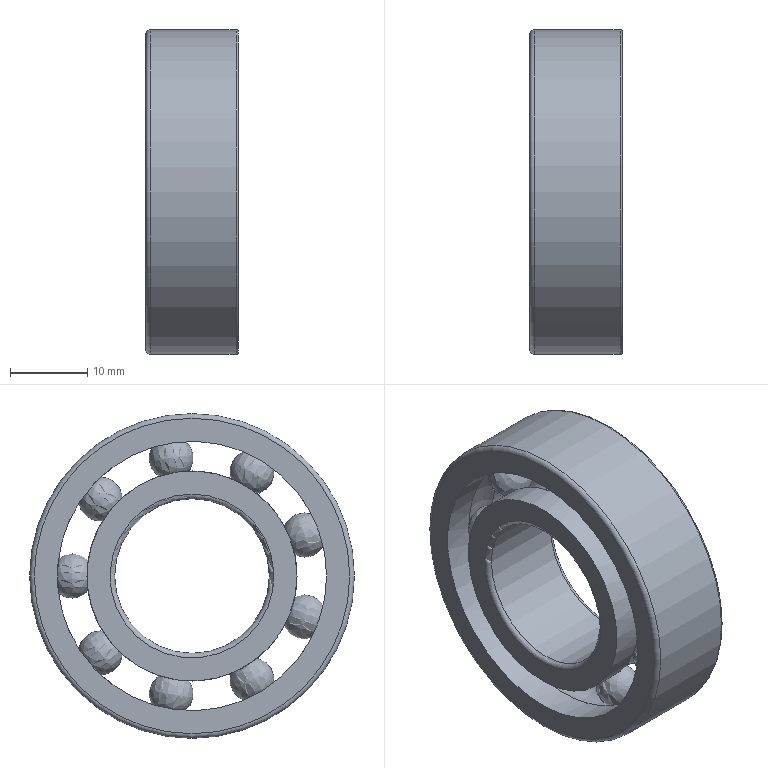Part | STEP file | Rolling bearing 70000C 7004 C GB_T 292 | 11 solids | 41 faces | box 12 x 42 x 42 mm | volume 8552 mm3 | torus 22 | sphere 9 | cylinder 5 | plane 4 | cone 1 | commonest cylinder face diameters 27.172 x2 20 x1 34.828 x1 42 x1
STEP:
#1=CARTESIAN_POINT('',(6.,13.712,-7.772));
#2=VERTEX_POINT('',#1);
#3=CARTESIAN_POINT('',(6.,10.035,-12.154));
#4=VERTEX_POINT('',#3);
#5=CARTESIAN_POINT('',(6.,11.874,-9.963));
#6=DIRECTION('',(0.,-0.766,0.6428));
#7=DIRECTION('',(-1.,0.,0.));
#8=AXIS2_PLACEMENT_3D('',#5,#6,#7);
#9=CIRCLE('',#8,2.86);
#10=EDGE_CURVE('',#2,#4,#9,.T.);
#11=ORIENTED_EDGE('',*,*,#10,.T.);
#12=ORIENTED_EDGE('',*,*,#10,.F.);
#13=EDGE_LOOP('',(#11,#12));
#14=FACE_OUTER_BOUND('',#13,.T.);
#15=CARTESIAN_POINT('',(3.875,10.407,-8.733));
#16=VERTEX_POINT('',#15);
#17=CARTESIAN_POINT('',(8.125,10.407,-8.733));
#18=VERTEX_POINT('',#17);
#19=CARTESIAN_POINT('',(6.,11.874,-9.963));
#20=DIRECTION('',(0.,0.6428,0.766));
#21=DIRECTION('',(0.,0.766,-0.6428));
#22=AXIS2_PLACEMENT_3D('',#19,#20,#21);
#23=CIRCLE('',#22,2.86);
#24=EDGE_CURVE('',#16,#18,#23,.T.);
#25=ORIENTED_EDGE('',*,*,#24,.T.);
#26=ORIENTED_EDGE('',*,*,#24,.F.);
#27=EDGE_LOOP('',(#25,#26));
#28=FACE_BOUND('',#27,.T.);
#29=CARTESIAN_POINT('',(8.125,13.34,-11.194));
#30=VERTEX_POINT('',#29);
#31=CARTESIAN_POINT('',(3.875,13.34,-11.194));
#32=VERTEX_POINT('',#31);
#33=CARTESIAN_POINT('',(6.,11.874,-9.963));
#34=DIRECTION('',(0.,0.6428,0.766));
#35=DIRECTION('',(0.,0.766,-0.6428));
#36=AXIS2_PLACEMENT_3D('',#33,#34,#35);
#37=CIRCLE('',#36,2.86);
#38=EDGE_CURVE('',#30,#32,#37,.T.);
#39=ORIENTED_EDGE('',*,*,#38,.T.);
#40=ORIENTED_EDGE('',*,*,#38,.F.);
#41=EDGE_LOOP('',(#39,#40));
#42=FACE_BOUND('',#41,.T.);
#43=CARTESIAN_POINT('',(6.,11.874,-9.963));
#44=DIRECTION('',(0.,0.6428,0.766));
#45=DIRECTION('',(1.,0.,0.));
#46=AXIS2_PLACEMENT_3D('',#43,#44,#45);
#47=SPHERICAL_SURFACE('',#46,2.86);
#48=ADVANCED_FACE('',(#14,#28,#42),#47,.T.);
#49=CLOSED_SHELL('',(#48));
#50=MANIFOLD_SOLID_BREP('',#49);
#51=CARTESIAN_POINT('',(6.,-10.227,11.993));
#52=VERTEX_POINT('',#51);
#53=CARTESIAN_POINT('',(6.,-5.273,14.853));
#54=VERTEX_POINT('',#53);
#55=CARTESIAN_POINT('',(6.,-7.75,13.423));
#56=DIRECTION('',(0.,0.5,-0.866));
#57=DIRECTION('',(-1.,0.,0.));
#58=AXIS2_PLACEMENT_3D('',#55,#56,#57);
#59=CIRCLE('',#58,2.86);
#60=EDGE_CURVE('',#52,#54,#59,.T.);
#61=ORIENTED_EDGE('',*,*,#60,.T.);
#62=ORIENTED_EDGE('',*,*,#60,.F.);
#63=EDGE_LOOP('',(#61,#62));
#64=FACE_OUTER_BOUND('',#63,.T.);
#65=CARTESIAN_POINT('',(3.875,-6.793,11.766));
#66=VERTEX_POINT('',#65);
#67=CARTESIAN_POINT('',(8.125,-6.793,11.766));
#68=VERTEX_POINT('',#67);
#69=CARTESIAN_POINT('',(6.,-7.75,13.423));
#70=DIRECTION('',(0.,-0.866,-0.5));
#71=DIRECTION('',(0.,-0.5,0.866));
#72=AXIS2_PLACEMENT_3D('',#69,#70,#71);
#73=CIRCLE('',#72,2.86);
#74=EDGE_CURVE('',#66,#68,#73,.T.);
#75=ORIENTED_EDGE('',*,*,#74,.T.);
#76=ORIENTED_EDGE('',*,*,#74,.F.);
#77=EDGE_LOOP('',(#75,#76));
#78=FACE_BOUND('',#77,.T.);
#79=CARTESIAN_POINT('',(8.125,-8.707,15.081));
#80=VERTEX_POINT('',#79);
#81=CARTESIAN_POINT('',(3.875,-8.707,15.081));
#82=VERTEX_POINT('',#81);
#83=CARTESIAN_POINT('',(6.,-7.75,13.423));
#84=DIRECTION('',(0.,-0.866,-0.5));
#85=DIRECTION('',(0.,-0.5,0.866));
#86=AXIS2_PLACEMENT_3D('',#83,#84,#85);
#87=CIRCLE('',#86,2.86);
#88=EDGE_CURVE('',#80,#82,#87,.T.);
#89=ORIENTED_EDGE('',*,*,#88,.T.);
#90=ORIENTED_EDGE('',*,*,#88,.F.);
#91=EDGE_LOOP('',(#89,#90));
#92=FACE_BOUND('',#91,.T.);
#93=CARTESIAN_POINT('',(6.,-7.75,13.423));
#94=DIRECTION('',(0.,-0.866,-0.5));
#95=DIRECTION('',(1.,0.,0.));
#96=AXIS2_PLACEMENT_3D('',#93,#94,#95);
#97=SPHERICAL_SURFACE('',#96,2.86);
#98=ADVANCED_FACE('',(#64,#78,#92),#97,.T.);
#99=CLOSED_SHELL('',(#98));
#100=MANIFOLD_SOLID_BREP('',#99);
#101=CARTESIAN_POINT('',(6.,-0.125,15.761));
#102=VERTEX_POINT('',#101);
#103=CARTESIAN_POINT('',(6.,5.508,14.768));
#104=VERTEX_POINT('',#103);
#105=CARTESIAN_POINT('',(6.,2.692,15.265));
#106=DIRECTION('',(0.,-0.1736,-0.9848));
#107=DIRECTION('',(-1.,0.,0.));
#108=AXIS2_PLACEMENT_3D('',#105,#106,#107);
#109=CIRCLE('',#108,2.86);
#110=EDGE_CURVE('',#102,#104,#109,.T.);
#111=ORIENTED_EDGE('',*,*,#110,.T.);
#112=ORIENTED_EDGE('',*,*,#110,.F.);
#113=EDGE_LOOP('',(#111,#112));
#114=FACE_OUTER_BOUND('',#113,.T.);
#115=CARTESIAN_POINT('',(3.875,2.359,13.38));
#116=VERTEX_POINT('',#115);
#117=CARTESIAN_POINT('',(8.125,2.359,13.38));
#118=VERTEX_POINT('',#117);
#119=CARTESIAN_POINT('',(6.,2.692,15.265));
#120=DIRECTION('',(0.,-0.9848,0.1736));
#121=DIRECTION('',(0.,0.1736,0.9848));
#122=AXIS2_PLACEMENT_3D('',#119,#120,#121);
#123=CIRCLE('',#122,2.86);
#124=EDGE_CURVE('',#116,#118,#123,.T.);
#125=ORIENTED_EDGE('',*,*,#124,.T.);
#126=ORIENTED_EDGE('',*,*,#124,.F.);
#127=EDGE_LOOP('',(#125,#126));
#128=FACE_BOUND('',#127,.T.);
#129=CARTESIAN_POINT('',(8.125,3.024,17.149));
#130=VERTEX_POINT('',#129);
#131=CARTESIAN_POINT('',(3.875,3.024,17.149));
#132=VERTEX_POINT('',#131);
#133=CARTESIAN_POINT('',(6.,2.692,15.265));
#134=DIRECTION('',(0.,-0.9848,0.1736));
#135=DIRECTION('',(0.,0.1736,0.9848));
#136=AXIS2_PLACEMENT_3D('',#133,#134,#135);
#137=CIRCLE('',#136,2.86);
#138=EDGE_CURVE('',#130,#132,#137,.T.);
#139=ORIENTED_EDGE('',*,*,#138,.T.);
#140=ORIENTED_EDGE('',*,*,#138,.F.);
#141=EDGE_LOOP('',(#139,#140));
#142=FACE_BOUND('',#141,.T.);
#143=CARTESIAN_POINT('',(6.,2.692,15.265));
#144=DIRECTION('',(0.,-0.9848,0.1736));
#145=DIRECTION('',(1.,0.,0.));
#146=AXIS2_PLACEMENT_3D('',#143,#144,#145);
#147=SPHERICAL_SURFACE('',#146,2.86);
#148=ADVANCED_FACE('',(#114,#128,#142),#147,.T.);
#149=CLOSED_SHELL('',(#148));
#150=MANIFOLD_SOLID_BREP('',#149);
#151=CARTESIAN_POINT('',(6.,-15.543,2.614));
#152=VERTEX_POINT('',#151);
#153=CARTESIAN_POINT('',(6.,-13.587,7.989));
#154=VERTEX_POINT('',#153);
#155=CARTESIAN_POINT('',(6.,-14.565,5.301));
#156=DIRECTION('',(0.,0.9397,-0.342));
#157=DIRECTION('',(-1.,0.,0.));
#158=AXIS2_PLACEMENT_3D('',#155,#156,#157);
#159=CIRCLE('',#158,2.86);
#160=EDGE_CURVE('',#152,#154,#159,.T.);
#161=ORIENTED_EDGE('',*,*,#160,.T.);
#162=ORIENTED_EDGE('',*,*,#160,.F.);
#163=EDGE_LOOP('',(#161,#162));
#164=FACE_OUTER_BOUND('',#163,.T.);
#165=CARTESIAN_POINT('',(3.875,-12.767,4.647));
#166=VERTEX_POINT('',#165);
#167=CARTESIAN_POINT('',(8.125,-12.767,4.647));
#168=VERTEX_POINT('',#167);
#169=CARTESIAN_POINT('',(6.,-14.565,5.301));
#170=DIRECTION('',(0.,-0.342,-0.9397));
#171=DIRECTION('',(0.,-0.9397,0.342));
#172=AXIS2_PLACEMENT_3D('',#169,#170,#171);
#173=CIRCLE('',#172,2.86);
#174=EDGE_CURVE('',#166,#168,#173,.T.);
#175=ORIENTED_EDGE('',*,*,#174,.T.);
#176=ORIENTED_EDGE('',*,*,#174,.F.);
#177=EDGE_LOOP('',(#175,#176));
#178=FACE_BOUND('',#177,.T.);
#179=CARTESIAN_POINT('',(8.125,-16.364,5.956));
#180=VERTEX_POINT('',#179);
#181=CARTESIAN_POINT('',(3.875,-16.364,5.956));
#182=VERTEX_POINT('',#181);
#183=CARTESIAN_POINT('',(6.,-14.565,5.301));
#184=DIRECTION('',(0.,-0.342,-0.9397));
#185=DIRECTION('',(0.,-0.9397,0.342));
#186=AXIS2_PLACEMENT_3D('',#183,#184,#185);
#187=CIRCLE('',#186,2.86);
#188=EDGE_CURVE('',#180,#182,#187,.T.);
#189=ORIENTED_EDGE('',*,*,#188,.T.);
#190=ORIENTED_EDGE('',*,*,#188,.F.);
#191=EDGE_LOOP('',(#189,#190));
#192=FACE_BOUND('',#191,.T.);
#193=CARTESIAN_POINT('',(6.,-14.565,5.301));
#194=DIRECTION('',(0.,-0.342,-0.9397));
#195=DIRECTION('',(1.,0.,0.));
#196=AXIS2_PLACEMENT_3D('',#193,#194,#195);
#197=SPHERICAL_SURFACE('',#196,2.86);
#198=ADVANCED_FACE('',(#164,#178,#192),#197,.T.);
#199=CLOSED_SHELL('',(#198));
#200=MANIFOLD_SOLID_BREP('',#199);
#201=CARTESIAN_POINT('',(6.,10.035,12.154));
#202=VERTEX_POINT('',#201);
#203=CARTESIAN_POINT('',(6.,13.712,7.772));
#204=VERTEX_POINT('',#203);
#205=CARTESIAN_POINT('',(6.,11.874,9.963));
#206=DIRECTION('',(0.,-0.766,-0.6428));
#207=DIRECTION('',(-1.,0.,0.));
#208=AXIS2_PLACEMENT_3D('',#205,#206,#207);
#209=CIRCLE('',#208,2.86);
#210=EDGE_CURVE('',#202,#204,#209,.T.);
#211=ORIENTED_EDGE('',*,*,#210,.T.);
#212=ORIENTED_EDGE('',*,*,#210,.F.);
#213=EDGE_LOOP('',(#211,#212));
#214=FACE_OUTER_BOUND('',#213,.T.);
#215=CARTESIAN_POINT('',(3.875,10.407,8.733));
#216=VERTEX_POINT('',#215);
#217=CARTESIAN_POINT('',(8.125,10.407,8.733));
#218=VERTEX_POINT('',#217);
#219=CARTESIAN_POINT('',(6.,11.874,9.963));
#220=DIRECTION('',(0.,-0.6428,0.766));
#221=DIRECTION('',(0.,0.766,0.6428));
#222=AXIS2_PLACEMENT_3D('',#219,#220,#221);
#223=CIRCLE('',#222,2.86);
#224=EDGE_CURVE('',#216,#218,#223,.T.);
#225=ORIENTED_EDGE('',*,*,#224,.T.);
#226=ORIENTED_EDGE('',*,*,#224,.F.);
#227=EDGE_LOOP('',(#225,#226));
#228=FACE_BOUND('',#227,.T.);
#229=CARTESIAN_POINT('',(8.125,13.34,11.194));
#230=VERTEX_POINT('',#229);
#231=CARTESIAN_POINT('',(3.875,13.34,11.194));
#232=VERTEX_POINT('',#231);
#233=CARTESIAN_POINT('',(6.,11.874,9.963));
#234=DIRECTION('',(0.,-0.6428,0.766));
#235=DIRECTION('',(0.,0.766,0.6428));
#236=AXIS2_PLACEMENT_3D('',#233,#234,#235);
#237=CIRCLE('',#236,2.86);
#238=EDGE_CURVE('',#230,#232,#237,.T.);
#239=ORIENTED_EDGE('',*,*,#238,.T.);
#240=ORIENTED_EDGE('',*,*,#238,.F.);
#241=EDGE_LOOP('',(#239,#240));
#242=FACE_BOUND('',#241,.T.);
#243=CARTESIAN_POINT('',(6.,11.874,9.963));
#244=DIRECTION('',(0.,-0.6428,0.766));
#245=DIRECTION('',(1.,0.,0.));
#246=AXIS2_PLACEMENT_3D('',#243,#244,#245);
#247=SPHERICAL_SURFACE('',#246,2.86);
#248=ADVANCED_FACE('',(#214,#228,#242),#247,.T.);
#249=CLOSED_SHELL('',(#248));
#250=MANIFOLD_SOLID_BREP('',#249);
#251=CARTESIAN_POINT('',(6.,-13.587,-7.989));
#252=VERTEX_POINT('',#251);
#253=CARTESIAN_POINT('',(6.,-15.543,-2.614));
#254=VERTEX_POINT('',#253);
#255=CARTESIAN_POINT('',(6.,-14.565,-5.301));
#256=DIRECTION('',(0.,0.9397,0.342));
#257=DIRECTION('',(-1.,0.,0.));
#258=AXIS2_PLACEMENT_3D('',#255,#256,#257);
#259=CIRCLE('',#258,2.86);
#260=EDGE_CURVE('',#252,#254,#259,.T.);
#261=ORIENTED_EDGE('',*,*,#260,.T.);
#262=ORIENTED_EDGE('',*,*,#260,.F.);
#263=EDGE_LOOP('',(#261,#262));
#264=FACE_OUTER_BOUND('',#263,.T.);
#265=CARTESIAN_POINT('',(3.875,-12.767,-4.647));
#266=VERTEX_POINT('',#265);
#267=CARTESIAN_POINT('',(8.125,-12.767,-4.647));
#268=VERTEX_POINT('',#267);
#269=CARTESIAN_POINT('',(6.,-14.565,-5.301));
#270=DIRECTION('',(0.,0.342,-0.9397));
#271=DIRECTION('',(0.,-0.9397,-0.342));
#272=AXIS2_PLACEMENT_3D('',#269,#270,#271);
#273=CIRCLE('',#272,2.86);
#274=EDGE_CURVE('',#266,#268,#273,.T.);
#275=ORIENTED_EDGE('',*,*,#274,.T.);
#276=ORIENTED_EDGE('',*,*,#274,.F.);
#277=EDGE_LOOP('',(#275,#276));
#278=FACE_BOUND('',#277,.T.);
#279=CARTESIAN_POINT('',(8.125,-16.364,-5.956));
#280=VERTEX_POINT('',#279);
#281=CARTESIAN_POINT('',(3.875,-16.364,-5.956));
#282=VERTEX_POINT('',#281);
#283=CARTESIAN_POINT('',(6.,-14.565,-5.301));
#284=DIRECTION('',(0.,0.342,-0.9397));
#285=DIRECTION('',(0.,-0.9397,-0.342));
#286=AXIS2_PLACEMENT_3D('',#283,#284,#285);
#287=CIRCLE('',#286,2.86);
#288=EDGE_CURVE('',#280,#282,#287,.T.);
#289=ORIENTED_EDGE('',*,*,#288,.T.);
#290=ORIENTED_EDGE('',*,*,#288,.F.);
#291=EDGE_LOOP('',(#289,#290));
#292=FACE_BOUND('',#291,.T.);
#293=CARTESIAN_POINT('',(6.,-14.565,-5.301));
#294=DIRECTION('',(0.,0.342,-0.9397));
#295=DIRECTION('',(1.,0.,0.));
#296=AXIS2_PLACEMENT_3D('',#293,#294,#295);
#297=SPHERICAL_SURFACE('',#296,2.86);
#298=ADVANCED_FACE('',(#264,#278,#292),#297,.T.);
#299=CLOSED_SHELL('',(#298));
#300=MANIFOLD_SOLID_BREP('',#299);
#301=CARTESIAN_POINT('',(6.,15.5,2.86));
#302=VERTEX_POINT('',#301);
#303=CARTESIAN_POINT('',(6.,15.5,-2.86));
#304=VERTEX_POINT('',#303);
#305=CARTESIAN_POINT('',(6.,15.5,0.));
#306=DIRECTION('',(0.,-1.,0.));
#307=DIRECTION('',(-1.,0.,0.));
#308=AXIS2_PLACEMENT_3D('',#305,#306,#307);
#309=CIRCLE('',#308,2.86);
#310=EDGE_CURVE('',#302,#304,#309,.T.);
#311=ORIENTED_EDGE('',*,*,#310,.T.);
#312=ORIENTED_EDGE('',*,*,#310,.F.);
#313=EDGE_LOOP('',(#311,#312));
#314=FACE_OUTER_BOUND('',#313,.T.);
#315=CARTESIAN_POINT('',(8.125,17.414,0.));
#316=VERTEX_POINT('',#315);
#317=CARTESIAN_POINT('',(3.875,17.414,0.));
#318=VERTEX_POINT('',#317);
#319=CARTESIAN_POINT('',(6.,15.5,0.));
#320=DIRECTION('',(0.,0.,1.));
#321=DIRECTION('',(0.,1.,0.));
#322=AXIS2_PLACEMENT_3D('',#319,#320,#321);
#323=CIRCLE('',#322,2.86);
#324=EDGE_CURVE('',#316,#318,#323,.T.);
#325=ORIENTED_EDGE('',*,*,#324,.T.);
#326=ORIENTED_EDGE('',*,*,#324,.F.);
#327=EDGE_LOOP('',(#325,#326));
#328=FACE_BOUND('',#327,.T.);
#329=CARTESIAN_POINT('',(3.875,13.586,0.));
#330=VERTEX_POINT('',#329);
#331=CARTESIAN_POINT('',(8.125,13.586,0.));
#332=VERTEX_POINT('',#331);
#333=CARTESIAN_POINT('',(6.,15.5,0.));
#334=DIRECTION('',(0.,0.,1.));
#335=DIRECTION('',(0.,1.,0.));
#336=AXIS2_PLACEMENT_3D('',#333,#334,#335);
#337=CIRCLE('',#336,2.86);
#338=EDGE_CURVE('',#330,#332,#337,.T.);
#339=ORIENTED_EDGE('',*,*,#338,.T.);
#340=ORIENTED_EDGE('',*,*,#338,.F.);
#341=EDGE_LOOP('',(#339,#340));
#342=FACE_BOUND('',#341,.T.);
#343=CARTESIAN_POINT('',(6.,15.5,0.));
#344=DIRECTION('',(0.,0.,1.));
#345=DIRECTION('',(1.,0.,0.));
#346=AXIS2_PLACEMENT_3D('',#343,#344,#345);
#347=SPHERICAL_SURFACE('',#346,2.86);
#348=ADVANCED_FACE('',(#314,#328,#342),#347,.T.);
#349=CLOSED_SHELL('',(#348));
#350=MANIFOLD_SOLID_BREP('',#349);
#351=CARTESIAN_POINT('',(6.,-5.273,-14.853));
#352=VERTEX_POINT('',#351);
#353=CARTESIAN_POINT('',(6.,-10.227,-11.993));
#354=VERTEX_POINT('',#353);
#355=CARTESIAN_POINT('',(6.,-7.75,-13.423));
#356=DIRECTION('',(0.,0.5,0.866));
#357=DIRECTION('',(-1.,0.,0.));
#358=AXIS2_PLACEMENT_3D('',#355,#356,#357);
#359=CIRCLE('',#358,2.86);
#360=EDGE_CURVE('',#352,#354,#359,.T.);
#361=ORIENTED_EDGE('',*,*,#360,.T.);
#362=ORIENTED_EDGE('',*,*,#360,.F.);
#363=EDGE_LOOP('',(#361,#362));
#364=FACE_OUTER_BOUND('',#363,.T.);
#365=CARTESIAN_POINT('',(3.875,-6.793,-11.766));
#366=VERTEX_POINT('',#365);
#367=CARTESIAN_POINT('',(8.125,-6.793,-11.766));
#368=VERTEX_POINT('',#367);
#369=CARTESIAN_POINT('',(6.,-7.75,-13.423));
#370=DIRECTION('',(0.,0.866,-0.5));
#371=DIRECTION('',(0.,-0.5,-0.866));
#372=AXIS2_PLACEMENT_3D('',#369,#370,#371);
#373=CIRCLE('',#372,2.86);
#374=EDGE_CURVE('',#366,#368,#373,.T.);
#375=ORIENTED_EDGE('',*,*,#374,.T.);
#376=ORIENTED_EDGE('',*,*,#374,.F.);
#377=EDGE_LOOP('',(#375,#376));
#378=FACE_BOUND('',#377,.T.);
#379=CARTESIAN_POINT('',(8.125,-8.707,-15.081));
#380=VERTEX_POINT('',#379);
#381=CARTESIAN_POINT('',(3.875,-8.707,-15.081));
#382=VERTEX_POINT('',#381);
#383=CARTESIAN_POINT('',(6.,-7.75,-13.423));
#384=DIRECTION('',(0.,0.866,-0.5));
#385=DIRECTION('',(0.,-0.5,-0.866));
#386=AXIS2_PLACEMENT_3D('',#383,#384,#385);
#387=CIRCLE('',#386,2.86);
#388=EDGE_CURVE('',#380,#382,#387,.T.);
#389=ORIENTED_EDGE('',*,*,#388,.T.);
#390=ORIENTED_EDGE('',*,*,#388,.F.);
#391=EDGE_LOOP('',(#389,#390));
#392=FACE_BOUND('',#391,.T.);
#393=CARTESIAN_POINT('',(6.,-7.75,-13.423));
#394=DIRECTION('',(0.,0.866,-0.5));
#395=DIRECTION('',(1.,0.,0.));
#396=AXIS2_PLACEMENT_3D('',#393,#394,#395);
#397=SPHERICAL_SURFACE('',#396,2.86);
#398=ADVANCED_FACE('',(#364,#378,#392),#397,.T.);
#399=CLOSED_SHELL('',(#398));
#400=MANIFOLD_SOLID_BREP('',#399);
#401=CARTESIAN_POINT('',(3.875,13.586,0.));
#402=VERTEX_POINT('',#401);
#403=CARTESIAN_POINT('',(3.875,10.407,8.733));
#404=VERTEX_POINT('',#403);
#405=CARTESIAN_POINT('',(3.875,0.,0.));
#406=DIRECTION('',(1.,0.,0.));
#407=DIRECTION('',(0.,1.,0.));
#408=AXIS2_PLACEMENT_3D('',#405,#406,#407);
#409=CIRCLE('',#408,13.586);
#410=EDGE_CURVE('',#402,#404,#409,.T.);
#411=ORIENTED_EDGE('',*,*,#410,.F.);
#412=CARTESIAN_POINT('',(3.875,10.407,-8.733));
#413=VERTEX_POINT('',#412);
#414=CARTESIAN_POINT('',(3.875,0.,0.));
#415=DIRECTION('',(1.,0.,0.));
#416=DIRECTION('',(0.,1.,0.));
#417=AXIS2_PLACEMENT_3D('',#414,#415,#416);
#418=CIRCLE('',#417,13.586);
#419=EDGE_CURVE('',#413,#402,#418,.T.);
#420=ORIENTED_EDGE('',*,*,#419,.F.);
#421=CARTESIAN_POINT('',(3.875,2.359,-13.38));
#422=VERTEX_POINT('',#421);
#423=CARTESIAN_POINT('',(3.875,0.,0.));
#424=DIRECTION('',(1.,0.,0.));
#425=DIRECTION('',(0.,1.,0.));
#426=AXIS2_PLACEMENT_3D('',#423,#424,#425);
#427=CIRCLE('',#426,13.586);
#428=EDGE_CURVE('',#422,#413,#427,.T.);
#429=ORIENTED_EDGE('',*,*,#428,.F.);
#430=CARTESIAN_POINT('',(3.875,-6.793,-11.766));
#431=VERTEX_POINT('',#430);
#432=CARTESIAN_POINT('',(3.875,0.,0.));
#433=DIRECTION('',(1.,0.,0.));
#434=DIRECTION('',(0.,1.,0.));
#435=AXIS2_PLACEMENT_3D('',#432,#433,#434);
#436=CIRCLE('',#435,13.586);
#437=EDGE_CURVE('',#431,#422,#436,.T.);
#438=ORIENTED_EDGE('',*,*,#437,.F.);
#439=CARTESIAN_POINT('',(3.875,-12.767,-4.647));
#440=VERTEX_POINT('',#439);
#441=CARTESIAN_POINT('',(3.875,0.,0.));
#442=DIRECTION('',(1.,0.,0.));
#443=DIRECTION('',(0.,1.,0.));
#444=AXIS2_PLACEMENT_3D('',#441,#442,#443);
#445=CIRCLE('',#444,13.586);
#446=EDGE_CURVE('',#440,#431,#445,.T.);
#447=ORIENTED_EDGE('',*,*,#446,.F.);
#448=CARTESIAN_POINT('',(3.875,-13.586,0.));
#449=VERTEX_POINT('',#448);
#450=CARTESIAN_POINT('',(3.875,0.,0.));
#451=DIRECTION('',(1.,0.,0.));
#452=DIRECTION('',(0.,1.,0.));
#453=AXIS2_PLACEMENT_3D('',#450,#451,#452);
#454=CIRCLE('',#453,13.586);
#455=EDGE_CURVE('',#449,#440,#454,.T.);
#456=ORIENTED_EDGE('',*,*,#455,.F.);
#457=CARTESIAN_POINT('',(0.,-13.586,0.));
#458=VERTEX_POINT('',#457);
#459=CARTESIAN_POINT('',(1.937,-13.586,0.));
#460=DIRECTION('',(-1.,0.,0.));
#461=VECTOR('',#460,13.586);
#462=LINE('',#459,#461);
#463=EDGE_CURVE('',#449,#458,#462,.T.);
#464=ORIENTED_EDGE('',*,*,#463,.T.);
#465=CARTESIAN_POINT('',(0.,0.,0.));
#466=DIRECTION('',(1.,0.,0.));
#467=DIRECTION('',(0.,1.,0.));
#468=AXIS2_PLACEMENT_3D('',#465,#466,#467);
#469=CIRCLE('',#468,13.586);
#470=EDGE_CURVE('',#458,#458,#469,.T.);
#471=ORIENTED_EDGE('',*,*,#470,.T.);
#472=ORIENTED_EDGE('',*,*,#463,.F.);
#473=CARTESIAN_POINT('',(3.875,-12.767,4.647));
#474=VERTEX_POINT('',#473);
#475=CARTESIAN_POINT('',(3.875,0.,0.));
#476=DIRECTION('',(1.,0.,0.));
#477=DIRECTION('',(0.,1.,0.));
#478=AXIS2_PLACEMENT_3D('',#475,#476,#477);
#479=CIRCLE('',#478,13.586);
#480=EDGE_CURVE('',#474,#449,#479,.T.);
#481=ORIENTED_EDGE('',*,*,#480,.F.);
#482=CARTESIAN_POINT('',(3.875,-6.793,11.766));
#483=VERTEX_POINT('',#482);
#484=CARTESIAN_POINT('',(3.875,0.,0.));
#485=DIRECTION('',(1.,0.,0.));
#486=DIRECTION('',(0.,1.,0.));
#487=AXIS2_PLACEMENT_3D('',#484,#485,#486);
#488=CIRCLE('',#487,13.586);
#489=EDGE_CURVE('',#483,#474,#488,.T.);
#490=ORIENTED_EDGE('',*,*,#489,.F.);
#491=CARTESIAN_POINT('',(3.875,2.359,13.38));
#492=VERTEX_POINT('',#491);
#493=CARTESIAN_POINT('',(3.875,0.,0.));
#494=DIRECTION('',(1.,0.,0.));
#495=DIRECTION('',(0.,1.,0.));
#496=AXIS2_PLACEMENT_3D('',#493,#494,#495);
#497=CIRCLE('',#496,13.586);
#498=EDGE_CURVE('',#492,#483,#497,.T.);
#499=ORIENTED_EDGE('',*,*,#498,.F.);
#500=CARTESIAN_POINT('',(3.875,0.,0.));
#501=DIRECTION('',(1.,0.,0.));
#502=DIRECTION('',(0.,1.,0.));
#503=AXIS2_PLACEMENT_3D('',#500,#501,#502);
#504=CIRCLE('',#503,13.586);
#505=EDGE_CURVE('',#404,#492,#504,.T.);
#506=ORIENTED_EDGE('',*,*,#505,.F.);
#507=EDGE_LOOP('',(#411,#420,#429,#438,#447,#456,#464,#471,#472,#481,#490,#499,#506));
#508=FACE_OUTER_BOUND('',#507,.T.);
#509=CARTESIAN_POINT('',(1.937,0.,0.));
#510=DIRECTION('',(1.,0.,0.));
#511=DIRECTION('',(0.,1.,0.));
#512=AXIS2_PLACEMENT_3D('',#509,#510,#511);
#513=CYLINDRICAL_SURFACE('',#512,13.586);
#514=ADVANCED_FACE('',(#508),#513,.T.);
#515=CARTESIAN_POINT('',(12.,-13.586,0.));
#516=VERTEX_POINT('',#515);
#517=CARTESIAN_POINT('',(12.,0.,0.));
#518=DIRECTION('',(1.,0.,0.));
#519=DIRECTION('',(0.,1.,0.));
#520=AXIS2_PLACEMENT_3D('',#517,#518,#519);
#521=CIRCLE('',#520,13.586);
#522=EDGE_CURVE('',#516,#516,#521,.T.);
#523=ORIENTED_EDGE('',*,*,#522,.F.);
#524=CARTESIAN_POINT('',(8.125,-13.586,0.));
#525=VERTEX_POINT('',#524);
#526=CARTESIAN_POINT('',(10.063,-13.586,0.));
#527=DIRECTION('',(-1.,0.,0.));
#528=VECTOR('',#527,13.586);
#529=LINE('',#526,#528);
#530=EDGE_CURVE('',#516,#525,#529,.T.);
#531=ORIENTED_EDGE('',*,*,#530,.T.);
#532=CARTESIAN_POINT('',(8.125,-12.767,-4.647));
#533=VERTEX_POINT('',#532);
#534=CARTESIAN_POINT('',(8.125,0.,0.));
#535=DIRECTION('',(1.,0.,0.));
#536=DIRECTION('',(0.,1.,0.));
#537=AXIS2_PLACEMENT_3D('',#534,#535,#536);
#538=CIRCLE('',#537,13.586);
#539=EDGE_CURVE('',#525,#533,#538,.T.);
#540=ORIENTED_EDGE('',*,*,#539,.T.);
#541=CARTESIAN_POINT('',(8.125,-6.793,-11.766));
#542=VERTEX_POINT('',#541);
#543=CARTESIAN_POINT('',(8.125,0.,0.));
#544=DIRECTION('',(1.,0.,0.));
#545=DIRECTION('',(0.,1.,0.));
#546=AXIS2_PLACEMENT_3D('',#543,#544,#545);
#547=CIRCLE('',#546,13.586);
#548=EDGE_CURVE('',#533,#542,#547,.T.);
#549=ORIENTED_EDGE('',*,*,#548,.T.);
#550=CARTESIAN_POINT('',(8.125,2.359,-13.38));
#551=VERTEX_POINT('',#550);
#552=CARTESIAN_POINT('',(8.125,0.,0.));
#553=DIRECTION('',(1.,0.,0.));
#554=DIRECTION('',(0.,1.,0.));
#555=AXIS2_PLACEMENT_3D('',#552,#553,#554);
#556=CIRCLE('',#555,13.586);
#557=EDGE_CURVE('',#542,#551,#556,.T.);
#558=ORIENTED_EDGE('',*,*,#557,.T.);
#559=CARTESIAN_POINT('',(8.125,10.407,-8.733));
#560=VERTEX_POINT('',#559);
#561=CARTESIAN_POINT('',(8.125,0.,0.));
#562=DIRECTION('',(1.,0.,0.));
#563=DIRECTION('',(0.,1.,0.));
#564=AXIS2_PLACEMENT_3D('',#561,#562,#563);
#565=CIRCLE('',#564,13.586);
#566=EDGE_CURVE('',#551,#560,#565,.T.);
#567=ORIENTED_EDGE('',*,*,#566,.T.);
#568=CARTESIAN_POINT('',(8.125,13.586,0.));
#569=VERTEX_POINT('',#568);
#570=CARTESIAN_POINT('',(8.125,0.,0.));
#571=DIRECTION('',(1.,0.,0.));
#572=DIRECTION('',(0.,1.,0.));
#573=AXIS2_PLACEMENT_3D('',#570,#571,#572);
#574=CIRCLE('',#573,13.586);
#575=EDGE_CURVE('',#560,#569,#574,.T.);
#576=ORIENTED_EDGE('',*,*,#575,.T.);
#577=CARTESIAN_POINT('',(8.125,10.407,8.733));
#578=VERTEX_POINT('',#577);
#579=CARTESIAN_POINT('',(8.125,0.,0.));
#580=DIRECTION('',(1.,0.,0.));
#581=DIRECTION('',(0.,1.,0.));
#582=AXIS2_PLACEMENT_3D('',#579,#580,#581);
#583=CIRCLE('',#582,13.586);
#584=EDGE_CURVE('',#569,#578,#583,.T.);
#585=ORIENTED_EDGE('',*,*,#584,.T.);
#586=CARTESIAN_POINT('',(8.125,2.359,13.38));
#587=VERTEX_POINT('',#586);
#588=CARTESIAN_POINT('',(8.125,0.,0.));
#589=DIRECTION('',(1.,0.,0.));
#590=DIRECTION('',(0.,1.,0.));
#591=AXIS2_PLACEMENT_3D('',#588,#589,#590);
#592=CIRCLE('',#591,13.586);
#593=EDGE_CURVE('',#578,#587,#592,.T.);
#594=ORIENTED_EDGE('',*,*,#593,.T.);
#595=CARTESIAN_POINT('',(8.125,-6.793,11.766));
#596=VERTEX_POINT('',#595);
#597=CARTESIAN_POINT('',(8.125,0.,0.));
#598=DIRECTION('',(1.,0.,0.));
#599=DIRECTION('',(0.,1.,0.));
#600=AXIS2_PLACEMENT_3D('',#597,#598,#599);
#601=CIRCLE('',#600,13.586);
#602=EDGE_CURVE('',#587,#596,#601,.T.);
#603=ORIENTED_EDGE('',*,*,#602,.T.);
#604=CARTESIAN_POINT('',(8.125,-12.767,4.647));
#605=VERTEX_POINT('',#604);
#606=CARTESIAN_POINT('',(8.125,0.,0.));
#607=DIRECTION('',(1.,0.,0.));
#608=DIRECTION('',(0.,1.,0.));
#609=AXIS2_PLACEMENT_3D('',#606,#607,#608);
#610=CIRCLE('',#609,13.586);
#611=EDGE_CURVE('',#596,#605,#610,.T.);
#612=ORIENTED_EDGE('',*,*,#611,.T.);
#613=CARTESIAN_POINT('',(8.125,0.,0.));
#614=DIRECTION('',(1.,0.,0.));
#615=DIRECTION('',(0.,1.,0.));
#616=AXIS2_PLACEMENT_3D('',#613,#614,#615);
#617=CIRCLE('',#616,13.586);
#618=EDGE_CURVE('',#605,#525,#617,.T.);
#619=ORIENTED_EDGE('',*,*,#618,.T.);
#620=ORIENTED_EDGE('',*,*,#530,.F.);
#621=EDGE_LOOP('',(#523,#531,#540,#549,#558,#567,#576,#585,#594,#603,#612,#619,#620));
#622=FACE_OUTER_BOUND('',#621,.T.);
#623=CARTESIAN_POINT('',(10.063,0.,0.));
#624=DIRECTION('',(1.,0.,0.));
#625=DIRECTION('',(0.,1.,0.));
#626=AXIS2_PLACEMENT_3D('',#623,#624,#625);
#627=CYLINDRICAL_SURFACE('',#626,13.586);
#628=ADVANCED_FACE('',(#622),#627,.T.);
#629=CARTESIAN_POINT('',(6.,11.874,-9.963));
#630=DIRECTION('',(0.,0.6428,0.766));
#631=DIRECTION('',(0.,0.766,-0.6428));
#632=AXIS2_PLACEMENT_3D('',#629,#630,#631);
#633=CIRCLE('',#632,2.86);
#634=EDGE_CURVE('',#413,#560,#633,.T.);
#635=ORIENTED_EDGE('',*,*,#634,.T.);
#636=ORIENTED_EDGE('',*,*,#566,.F.);
#637=CARTESIAN_POINT('',(6.,2.692,-15.265));
#638=DIRECTION('',(0.,0.9848,0.1736));
#639=DIRECTION('',(0.,0.1736,-0.9848));
#640=AXIS2_PLACEMENT_3D('',#637,#638,#639);
#641=CIRCLE('',#640,2.86);
#642=EDGE_CURVE('',#422,#551,#641,.T.);
#643=ORIENTED_EDGE('',*,*,#642,.F.);
#644=ORIENTED_EDGE('',*,*,#428,.T.);
#645=EDGE_LOOP('',(#635,#636,#643,#644));
#646=FACE_OUTER_BOUND('',#645,.T.);
#647=CARTESIAN_POINT('',(6.,0.,0.));
#648=DIRECTION('',(1.,0.,0.));
#649=DIRECTION('',(0.,0.,-1.));
#650=AXIS2_PLACEMENT_3D('',#647,#648,#649);
#651=TOROIDAL_SURFACE('',#650,15.5,2.86);
#652=ADVANCED_FACE('',(#646),#651,.F.);
#653=ORIENTED_EDGE('',*,*,#522,.T.);
#654=EDGE_LOOP('',(#653));
#655=FACE_OUTER_BOUND('',#654,.T.);
#656=CARTESIAN_POINT('',(12.,0.,10.6));
#657=VERTEX_POINT('',#656);
#658=CARTESIAN_POINT('',(12.,0.,0.));
#659=DIRECTION('',(1.,0.,0.));
#660=DIRECTION('',(0.,-1.,0.));
#661=AXIS2_PLACEMENT_3D('',#658,#659,#660);
#662=CIRCLE('',#661,10.6);
#663=EDGE_CURVE('',#657,#657,#662,.T.);
#664=ORIENTED_EDGE('',*,*,#663,.F.);
#665=EDGE_LOOP('',(#664));
#666=FACE_BOUND('',#665,.T.);
#667=CARTESIAN_POINT('',(12.,11.793,0.));
#668=DIRECTION('',(1.,0.,0.));
#669=DIRECTION('',(0.,0.,-1.));
#670=AXIS2_PLACEMENT_3D('',#667,#668,#669);
#671=PLANE('',#670);
#672=ADVANCED_FACE('',(#655,#666),#671,.T.);
#673=CARTESIAN_POINT('',(11.4,0.,10.));
#674=VERTEX_POINT('',#673);
#675=CARTESIAN_POINT('',(11.4,-10.,0.));
#676=VERTEX_POINT('',#675);
#677=CARTESIAN_POINT('',(11.4,0.,0.));
#678=DIRECTION('',(-1.,0.,0.));
#679=DIRECTION('',(0.,-1.,0.));
#680=AXIS2_PLACEMENT_3D('',#677,#678,#679);
#681=CIRCLE('',#680,10.);
#682=EDGE_CURVE('',#674,#676,#681,.T.);
#683=ORIENTED_EDGE('',*,*,#682,.T.);
#684=CARTESIAN_POINT('',(11.4,0.,0.));
#685=DIRECTION('',(-1.,0.,0.));
#686=DIRECTION('',(0.,-1.,0.));
#687=AXIS2_PLACEMENT_3D('',#684,#685,#686);
#688=CIRCLE('',#687,10.);
#689=EDGE_CURVE('',#676,#674,#688,.T.);
#690=ORIENTED_EDGE('',*,*,#689,.T.);
#691=CARTESIAN_POINT('',(11.4,0.,10.6));
#692=DIRECTION('',(0.,-1.,0.));
#693=DIRECTION('',(0.,0.,1.));
#694=AXIS2_PLACEMENT_3D('',#691,#692,#693);
#695=CIRCLE('',#694,0.6);
#696=EDGE_CURVE('',#674,#657,#695,.T.);
#697=ORIENTED_EDGE('',*,*,#696,.T.);
#698=ORIENTED_EDGE('',*,*,#663,.T.);
#699=ORIENTED_EDGE('',*,*,#696,.F.);
#700=EDGE_LOOP('',(#683,#690,#697,#698,#699));
#701=FACE_OUTER_BOUND('',#700,.T.);
#702=CARTESIAN_POINT('',(11.4,0.,0.));
#703=DIRECTION('',(1.,0.,0.));
#704=DIRECTION('',(0.,0.,-1.));
#705=AXIS2_PLACEMENT_3D('',#702,#703,#704);
#706=TOROIDAL_SURFACE('',#705,10.6,0.6);
#707=ADVANCED_FACE('',(#701),#706,.T.);
#708=ORIENTED_EDGE('',*,*,#470,.F.);
#709=EDGE_LOOP('',(#708));
#710=FACE_OUTER_BOUND('',#709,.T.);
#711=CARTESIAN_POINT('',(0.,0.,10.6));
#712=VERTEX_POINT('',#711);
#713=CARTESIAN_POINT('',(0.,0.,0.));
#714=DIRECTION('',(-1.,0.,0.));
#715=DIRECTION('',(0.,-1.,0.));
#716=AXIS2_PLACEMENT_3D('',#713,#714,#715);
#717=CIRCLE('',#716,10.6);
#718=EDGE_CURVE('',#712,#712,#717,.T.);
#719=ORIENTED_EDGE('',*,*,#718,.F.);
#720=EDGE_LOOP('',(#719));
#721=FACE_BOUND('',#720,.T.);
#722=CARTESIAN_POINT('',(0.,11.793,0.));
#723=DIRECTION('',(-1.,0.,0.));
#724=DIRECTION('',(0.,0.,1.));
#725=AXIS2_PLACEMENT_3D('',#722,#723,#724);
#726=PLANE('',#725);
#727=ADVANCED_FACE('',(#710,#721),#726,.T.);
#728=ORIENTED_EDGE('',*,*,#682,.F.);
#729=ORIENTED_EDGE('',*,*,#689,.F.);
#730=CARTESIAN_POINT('',(0.6,-10.,0.));
#731=VERTEX_POINT('',#730);
#732=CARTESIAN_POINT('',(6.,-10.,0.));
#733=DIRECTION('',(-1.,0.,0.));
#734=VECTOR('',#733,10.);
#735=LINE('',#732,#734);
#736=EDGE_CURVE('',#676,#731,#735,.T.);
#737=ORIENTED_EDGE('',*,*,#736,.T.);
#738=CARTESIAN_POINT('',(0.6,0.,10.));
#739=VERTEX_POINT('',#738);
#740=CARTESIAN_POINT('',(0.6,0.,0.));
#741=DIRECTION('',(1.,0.,0.));
#742=DIRECTION('',(0.,-1.,0.));
#743=AXIS2_PLACEMENT_3D('',#740,#741,#742);
#744=CIRCLE('',#743,10.);
#745=EDGE_CURVE('',#739,#731,#744,.T.);
#746=ORIENTED_EDGE('',*,*,#745,.F.);
#747=CARTESIAN_POINT('',(0.6,0.,0.));
#748=DIRECTION('',(1.,0.,0.));
#749=DIRECTION('',(0.,-1.,0.));
#750=AXIS2_PLACEMENT_3D('',#747,#748,#749);
#751=CIRCLE('',#750,10.);
#752=EDGE_CURVE('',#731,#739,#751,.T.);
#753=ORIENTED_EDGE('',*,*,#752,.F.);
#754=ORIENTED_EDGE('',*,*,#736,.F.);
#755=EDGE_LOOP('',(#728,#729,#737,#746,#753,#754));
#756=FACE_OUTER_BOUND('',#755,.T.);
#757=CARTESIAN_POINT('',(6.,0.,0.));
#758=DIRECTION('',(1.,0.,0.));
#759=DIRECTION('',(0.,1.,0.));
#760=AXIS2_PLACEMENT_3D('',#757,#758,#759);
#761=CYLINDRICAL_SURFACE('',#760,10.);
#762=ADVANCED_FACE('',(#756),#761,.F.);
#763=ORIENTED_EDGE('',*,*,#718,.T.);
#764=CARTESIAN_POINT('',(0.6,0.,10.6));
#765=DIRECTION('',(0.,-1.,0.));
#766=DIRECTION('',(0.,0.,1.));
#767=AXIS2_PLACEMENT_3D('',#764,#765,#766);
#768=CIRCLE('',#767,0.6);
#769=EDGE_CURVE('',#712,#739,#768,.T.);
#770=ORIENTED_EDGE('',*,*,#769,.T.);
#771=ORIENTED_EDGE('',*,*,#745,.T.);
#772=ORIENTED_EDGE('',*,*,#752,.T.);
#773=ORIENTED_EDGE('',*,*,#769,.F.);
#774=EDGE_LOOP('',(#763,#770,#771,#772,#773));
#775=FACE_OUTER_BOUND('',#774,.T.);
#776=CARTESIAN_POINT('',(0.6,0.,0.));
#777=DIRECTION('',(1.,0.,0.));
#778=DIRECTION('',(0.,0.,-1.));
#779=AXIS2_PLACEMENT_3D('',#776,#777,#778);
#780=TOROIDAL_SURFACE('',#779,10.6,0.6);
#781=ADVANCED_FACE('',(#775),#780,.T.);
#782=ORIENTED_EDGE('',*,*,#634,.F.);
#783=ORIENTED_EDGE('',*,*,#419,.T.);
#784=CARTESIAN_POINT('',(6.,15.5,0.));
#785=DIRECTION('',(0.,0.,1.));
#786=DIRECTION('',(0.,1.,0.));
#787=AXIS2_PLACEMENT_3D('',#784,#785,#786);
#788=CIRCLE('',#787,2.86);
#789=EDGE_CURVE('',#402,#569,#788,.T.);
#790=ORIENTED_EDGE('',*,*,#789,.T.);
#791=ORIENTED_EDGE('',*,*,#575,.F.);
#792=EDGE_LOOP('',(#782,#783,#790,#791));
#793=FACE_OUTER_BOUND('',#792,.T.);
#794=CARTESIAN_POINT('',(6.,0.,0.));
#795=DIRECTION('',(1.,0.,0.));
#796=DIRECTION('',(0.,0.,-1.));
#797=AXIS2_PLACEMENT_3D('',#794,#795,#796);
#798=TOROIDAL_SURFACE('',#797,15.5,2.86);
#799=ADVANCED_FACE('',(#793),#798,.F.);
#800=ORIENTED_EDGE('',*,*,#642,.T.);
#801=ORIENTED_EDGE('',*,*,#557,.F.);
#802=CARTESIAN_POINT('',(6.,-7.75,-13.423));
#803=DIRECTION('',(0.,0.866,-0.5));
#804=DIRECTION('',(0.,-0.5,-0.866));
#805=AXIS2_PLACEMENT_3D('',#802,#803,#804);
#806=CIRCLE('',#805,2.86);
#807=EDGE_CURVE('',#431,#542,#806,.T.);
#808=ORIENTED_EDGE('',*,*,#807,.F.);
#809=ORIENTED_EDGE('',*,*,#437,.T.);
#810=EDGE_LOOP('',(#800,#801,#808,#809));
#811=FACE_OUTER_BOUND('',#810,.T.);
#812=CARTESIAN_POINT('',(6.,0.,0.));
#813=DIRECTION('',(1.,0.,0.));
#814=DIRECTION('',(0.,0.,-1.));
#815=AXIS2_PLACEMENT_3D('',#812,#813,#814);
#816=TOROIDAL_SURFACE('',#815,15.5,2.86);
#817=ADVANCED_FACE('',(#811),#816,.F.);
#818=ORIENTED_EDGE('',*,*,#807,.T.);
#819=ORIENTED_EDGE('',*,*,#548,.F.);
#820=CARTESIAN_POINT('',(6.,-14.565,-5.301));
#821=DIRECTION('',(0.,0.342,-0.9397));
#822=DIRECTION('',(0.,-0.9397,-0.342));
#823=AXIS2_PLACEMENT_3D('',#820,#821,#822);
#824=CIRCLE('',#823,2.86);
#825=EDGE_CURVE('',#440,#533,#824,.T.);
#826=ORIENTED_EDGE('',*,*,#825,.F.);
#827=ORIENTED_EDGE('',*,*,#446,.T.);
#828=EDGE_LOOP('',(#818,#819,#826,#827));
#829=FACE_OUTER_BOUND('',#828,.T.);
#830=CARTESIAN_POINT('',(6.,0.,0.));
#831=DIRECTION('',(1.,0.,0.));
#832=DIRECTION('',(0.,0.,-1.));
#833=AXIS2_PLACEMENT_3D('',#830,#831,#832);
#834=TOROIDAL_SURFACE('',#833,15.5,2.86);
#835=ADVANCED_FACE('',(#829),#834,.F.);
#836=ORIENTED_EDGE('',*,*,#825,.T.);
#837=ORIENTED_EDGE('',*,*,#539,.F.);
#838=ORIENTED_EDGE('',*,*,#618,.F.);
#839=CARTESIAN_POINT('',(6.,-14.565,5.301));
#840=DIRECTION('',(0.,-0.342,-0.9397));
#841=DIRECTION('',(0.,-0.9397,0.342));
#842=AXIS2_PLACEMENT_3D('',#839,#840,#841);
#843=CIRCLE('',#842,2.86);
#844=EDGE_CURVE('',#474,#605,#843,.T.);
#845=ORIENTED_EDGE('',*,*,#844,.F.);
#846=ORIENTED_EDGE('',*,*,#480,.T.);
#847=ORIENTED_EDGE('',*,*,#455,.T.);
#848=EDGE_LOOP('',(#836,#837,#838,#845,#846,#847));
#849=FACE_OUTER_BOUND('',#848,.T.);
#850=CARTESIAN_POINT('',(6.,0.,0.));
#851=DIRECTION('',(1.,0.,0.));
#852=DIRECTION('',(0.,0.,-1.));
#853=AXIS2_PLACEMENT_3D('',#850,#851,#852);
#854=TOROIDAL_SURFACE('',#853,15.5,2.86);
#855=ADVANCED_FACE('',(#849),#854,.F.);
#856=ORIENTED_EDGE('',*,*,#844,.T.);
#857=ORIENTED_EDGE('',*,*,#611,.F.);
#858=CARTESIAN_POINT('',(6.,-7.75,13.423));
#859=DIRECTION('',(0.,-0.866,-0.5));
#860=DIRECTION('',(0.,-0.5,0.866));
#861=AXIS2_PLACEMENT_3D('',#858,#859,#860);
#862=CIRCLE('',#861,2.86);
#863=EDGE_CURVE('',#483,#596,#862,.T.);
#864=ORIENTED_EDGE('',*,*,#863,.F.);
#865=ORIENTED_EDGE('',*,*,#489,.T.);
#866=EDGE_LOOP('',(#856,#857,#864,#865));
#867=FACE_OUTER_BOUND('',#866,.T.);
#868=CARTESIAN_POINT('',(6.,0.,0.));
#869=DIRECTION('',(1.,0.,0.));
#870=DIRECTION('',(0.,0.,-1.));
#871=AXIS2_PLACEMENT_3D('',#868,#869,#870);
#872=TOROIDAL_SURFACE('',#871,15.5,2.86);
#873=ADVANCED_FACE('',(#867),#872,.F.);
#874=ORIENTED_EDGE('',*,*,#863,.T.);
#875=ORIENTED_EDGE('',*,*,#602,.F.);
#876=CARTESIAN_POINT('',(6.,2.692,15.265));
#877=DIRECTION('',(0.,-0.9848,0.1736));
#878=DIRECTION('',(0.,0.1736,0.9848));
#879=AXIS2_PLACEMENT_3D('',#876,#877,#878);
#880=CIRCLE('',#879,2.86);
#881=EDGE_CURVE('',#492,#587,#880,.T.);
#882=ORIENTED_EDGE('',*,*,#881,.F.);
#883=ORIENTED_EDGE('',*,*,#498,.T.);
#884=EDGE_LOOP('',(#874,#875,#882,#883));
#885=FACE_OUTER_BOUND('',#884,.T.);
#886=CARTESIAN_POINT('',(6.,0.,0.));
#887=DIRECTION('',(1.,0.,0.));
#888=DIRECTION('',(0.,-0.1736,0.9848));
#889=AXIS2_PLACEMENT_3D('',#886,#887,#888);
#890=TOROIDAL_SURFACE('',#889,15.5,2.86);
#891=ADVANCED_FACE('',(#885),#890,.F.);
#892=ORIENTED_EDGE('',*,*,#881,.T.);
#893=ORIENTED_EDGE('',*,*,#593,.F.);
#894=CARTESIAN_POINT('',(6.,11.874,9.963));
#895=DIRECTION('',(0.,-0.6428,0.766));
#896=DIRECTION('',(0.,0.766,0.6428));
#897=AXIS2_PLACEMENT_3D('',#894,#895,#896);
#898=CIRCLE('',#897,2.86);
#899=EDGE_CURVE('',#404,#578,#898,.T.);
#900=ORIENTED_EDGE('',*,*,#899,.F.);
#901=ORIENTED_EDGE('',*,*,#505,.T.);
#902=EDGE_LOOP('',(#892,#893,#900,#901));
#903=FACE_OUTER_BOUND('',#902,.T.);
#904=CARTESIAN_POINT('',(6.,0.,0.));
#905=DIRECTION('',(1.,0.,0.));
#906=DIRECTION('',(0.,0.,-1.));
#907=AXIS2_PLACEMENT_3D('',#904,#905,#906);
#908=TOROIDAL_SURFACE('',#907,15.5,2.86);
#909=ADVANCED_FACE('',(#903),#908,.F.);
#910=ORIENTED_EDGE('',*,*,#899,.T.);
#911=ORIENTED_EDGE('',*,*,#584,.F.);
#912=ORIENTED_EDGE('',*,*,#789,.F.);
#913=ORIENTED_EDGE('',*,*,#410,.T.);
#914=EDGE_LOOP('',(#910,#911,#912,#913));
#915=FACE_OUTER_BOUND('',#914,.T.);
#916=CARTESIAN_POINT('',(6.,0.,0.));
#917=DIRECTION('',(1.,0.,0.));
#918=DIRECTION('',(0.,0.,-1.));
#919=AXIS2_PLACEMENT_3D('',#916,#917,#918);
#920=TOROIDAL_SURFACE('',#919,15.5,2.86);
#921=ADVANCED_FACE('',(#915),#920,.F.);
#922=CLOSED_SHELL('',(#514,#628,#652,#672,#707,#727,#762,#781,#799,#817,#835,#855,#873,#891,#909,#921));
#923=MANIFOLD_SOLID_BREP('',#922);
#924=CARTESIAN_POINT('',(6.,5.508,-14.768));
#925=VERTEX_POINT('',#924);
#926=CARTESIAN_POINT('',(6.,-0.125,-15.761));
#927=VERTEX_POINT('',#926);
#928=CARTESIAN_POINT('',(6.,2.692,-15.265));
#929=DIRECTION('',(0.,-0.1736,0.9848));
#930=DIRECTION('',(-1.,0.,0.));
#931=AXIS2_PLACEMENT_3D('',#928,#929,#930);
#932=CIRCLE('',#931,2.86);
#933=EDGE_CURVE('',#925,#927,#932,.T.);
#934=ORIENTED_EDGE('',*,*,#933,.T.);
#935=ORIENTED_EDGE('',*,*,#933,.F.);
#936=EDGE_LOOP('',(#934,#935));
#937=FACE_OUTER_BOUND('',#936,.T.);
#938=CARTESIAN_POINT('',(3.875,2.359,-13.38));
#939=VERTEX_POINT('',#938);
#940=CARTESIAN_POINT('',(8.125,2.359,-13.38));
#941=VERTEX_POINT('',#940);
#942=CARTESIAN_POINT('',(6.,2.692,-15.265));
#943=DIRECTION('',(0.,0.9848,0.1736));
#944=DIRECTION('',(0.,0.1736,-0.9848));
#945=AXIS2_PLACEMENT_3D('',#942,#943,#944);
#946=CIRCLE('',#945,2.86);
#947=EDGE_CURVE('',#939,#941,#946,.T.);
#948=ORIENTED_EDGE('',*,*,#947,.T.);
#949=ORIENTED_EDGE('',*,*,#947,.F.);
#950=EDGE_LOOP('',(#948,#949));
#951=FACE_BOUND('',#950,.T.);
#952=CARTESIAN_POINT('',(8.125,3.024,-17.149));
#953=VERTEX_POINT('',#952);
#954=CARTESIAN_POINT('',(3.875,3.024,-17.149));
#955=VERTEX_POINT('',#954);
#956=CARTESIAN_POINT('',(6.,2.692,-15.265));
#957=DIRECTION('',(0.,0.9848,0.1736));
#958=DIRECTION('',(0.,0.1736,-0.9848));
#959=AXIS2_PLACEMENT_3D('',#956,#957,#958);
#960=CIRCLE('',#959,2.86);
#961=EDGE_CURVE('',#953,#955,#960,.T.);
#962=ORIENTED_EDGE('',*,*,#961,.T.);
#963=ORIENTED_EDGE('',*,*,#961,.F.);
#964=EDGE_LOOP('',(#962,#963));
#965=FACE_BOUND('',#964,.T.);
#966=CARTESIAN_POINT('',(6.,2.692,-15.265));
#967=DIRECTION('',(0.,0.9848,0.1736));
#968=DIRECTION('',(1.,0.,0.));
#969=AXIS2_PLACEMENT_3D('',#966,#967,#968);
#970=SPHERICAL_SURFACE('',#969,2.86);
#971=ADVANCED_FACE('',(#937,#951,#965),#970,.T.);
#972=CLOSED_SHELL('',(#971));
#973=MANIFOLD_SOLID_BREP('',#972);
#974=CARTESIAN_POINT('',(12.,-18.097,0.));
#975=VERTEX_POINT('',#974);
#976=CARTESIAN_POINT('',(12.,0.,0.));
#977=DIRECTION('',(1.,0.,0.));
#978=DIRECTION('',(0.,1.,0.));
#979=AXIS2_PLACEMENT_3D('',#976,#977,#978);
#980=CIRCLE('',#979,18.097);
#981=EDGE_CURVE('',#975,#975,#980,.T.);
#982=ORIENTED_EDGE('',*,*,#981,.T.);
#983=CARTESIAN_POINT('',(8.125,-17.414,0.));
#984=VERTEX_POINT('',#983);
#985=CARTESIAN_POINT('',(10.063,-17.756,0.));
#986=DIRECTION('',(-0.9848,0.1736,0.));
#987=VECTOR('',#986,17.756);
#988=LINE('',#985,#987);
#989=EDGE_CURVE('',#975,#984,#988,.T.);
#990=ORIENTED_EDGE('',*,*,#989,.T.);
#991=CARTESIAN_POINT('',(8.125,-16.364,5.956));
#992=VERTEX_POINT('',#991);
#993=CARTESIAN_POINT('',(8.125,0.,0.));
#994=DIRECTION('',(1.,0.,0.));
#995=DIRECTION('',(0.,1.,0.));
#996=AXIS2_PLACEMENT_3D('',#993,#994,#995);
#997=CIRCLE('',#996,17.414);
#998=EDGE_CURVE('',#992,#984,#997,.T.);
#999=ORIENTED_EDGE('',*,*,#998,.F.);
#1000=CARTESIAN_POINT('',(8.125,-8.707,15.081));
#1001=VERTEX_POINT('',#1000);
#1002=CARTESIAN_POINT('',(8.125,0.,0.));
#1003=DIRECTION('',(1.,0.,0.));
#1004=DIRECTION('',(0.,1.,0.));
#1005=AXIS2_PLACEMENT_3D('',#1002,#1003,#1004);
#1006=CIRCLE('',#1005,17.414);
#1007=EDGE_CURVE('',#1001,#992,#1006,.T.);
#1008=ORIENTED_EDGE('',*,*,#1007,.F.);
#1009=CARTESIAN_POINT('',(8.125,3.024,17.149));
#1010=VERTEX_POINT('',#1009);
#1011=CARTESIAN_POINT('',(8.125,0.,0.));
#1012=DIRECTION('',(1.,0.,0.));
#1013=DIRECTION('',(0.,1.,0.));
#1014=AXIS2_PLACEMENT_3D('',#1011,#1012,#1013);
#1015=CIRCLE('',#1014,17.414);
#1016=EDGE_CURVE('',#1010,#1001,#1015,.T.);
#1017=ORIENTED_EDGE('',*,*,#1016,.F.);
#1018=CARTESIAN_POINT('',(8.125,13.34,11.194));
#1019=VERTEX_POINT('',#1018);
#1020=CARTESIAN_POINT('',(8.125,0.,0.));
#1021=DIRECTION('',(1.,0.,0.));
#1022=DIRECTION('',(0.,1.,0.));
#1023=AXIS2_PLACEMENT_3D('',#1020,#1021,#1022);
#1024=CIRCLE('',#1023,17.414);
#1025=EDGE_CURVE('',#1019,#1010,#1024,.T.);
#1026=ORIENTED_EDGE('',*,*,#1025,.F.);
#1027=CARTESIAN_POINT('',(8.125,17.414,0.));
#1028=VERTEX_POINT('',#1027);
#1029=CARTESIAN_POINT('',(8.125,0.,0.));
#1030=DIRECTION('',(1.,0.,0.));
#1031=DIRECTION('',(0.,1.,0.));
#1032=AXIS2_PLACEMENT_3D('',#1029,#1030,#1031);
#1033=CIRCLE('',#1032,17.414);
#1034=EDGE_CURVE('',#1028,#1019,#1033,.T.);
#1035=ORIENTED_EDGE('',*,*,#1034,.F.);
#1036=CARTESIAN_POINT('',(8.125,13.34,-11.194));
#1037=VERTEX_POINT('',#1036);
#1038=CARTESIAN_POINT('',(8.125,0.,0.));
#1039=DIRECTION('',(1.,0.,0.));
#1040=DIRECTION('',(0.,1.,0.));
#1041=AXIS2_PLACEMENT_3D('',#1038,#1039,#1040);
#1042=CIRCLE('',#1041,17.414);
#1043=EDGE_CURVE('',#1037,#1028,#1042,.T.);
#1044=ORIENTED_EDGE('',*,*,#1043,.F.);
#1045=CARTESIAN_POINT('',(8.125,3.024,-17.149));
#1046=VERTEX_POINT('',#1045);
#1047=CARTESIAN_POINT('',(8.125,0.,0.));
#1048=DIRECTION('',(1.,0.,0.));
#1049=DIRECTION('',(0.,1.,0.));
#1050=AXIS2_PLACEMENT_3D('',#1047,#1048,#1049);
#1051=CIRCLE('',#1050,17.414);
#1052=EDGE_CURVE('',#1046,#1037,#1051,.T.);
#1053=ORIENTED_EDGE('',*,*,#1052,.F.);
#1054=CARTESIAN_POINT('',(8.125,-8.707,-15.081));
#1055=VERTEX_POINT('',#1054);
#1056=CARTESIAN_POINT('',(8.125,0.,0.));
#1057=DIRECTION('',(1.,0.,0.));
#1058=DIRECTION('',(0.,1.,0.));
#1059=AXIS2_PLACEMENT_3D('',#1056,#1057,#1058);
#1060=CIRCLE('',#1059,17.414);
#1061=EDGE_CURVE('',#1055,#1046,#1060,.T.);
#1062=ORIENTED_EDGE('',*,*,#1061,.F.);
#1063=CARTESIAN_POINT('',(8.125,-16.364,-5.956));
#1064=VERTEX_POINT('',#1063);
#1065=CARTESIAN_POINT('',(8.125,0.,0.));
#1066=DIRECTION('',(1.,0.,0.));
#1067=DIRECTION('',(0.,1.,0.));
#1068=AXIS2_PLACEMENT_3D('',#1065,#1066,#1067);
#1069=CIRCLE('',#1068,17.414);
#1070=EDGE_CURVE('',#1064,#1055,#1069,.T.);
#1071=ORIENTED_EDGE('',*,*,#1070,.F.);
#1072=CARTESIAN_POINT('',(8.125,0.,0.));
#1073=DIRECTION('',(1.,0.,0.));
#1074=DIRECTION('',(0.,1.,0.));
#1075=AXIS2_PLACEMENT_3D('',#1072,#1073,#1074);
#1076=CIRCLE('',#1075,17.414);
#1077=EDGE_CURVE('',#984,#1064,#1076,.T.);
#1078=ORIENTED_EDGE('',*,*,#1077,.F.);
#1079=ORIENTED_EDGE('',*,*,#989,.F.);
#1080=EDGE_LOOP('',(#982,#990,#999,#1008,#1017,#1026,#1035,#1044,#1053,#1062,#1071,#1078,#1079));
#1081=FACE_OUTER_BOUND('',#1080,.T.);
#1082=CARTESIAN_POINT('',(10.063,0.,0.));
#1083=DIRECTION('',(1.,0.,0.));
#1084=DIRECTION('',(0.,1.,0.));
#1085=AXIS2_PLACEMENT_3D('',#1082,#1083,#1084);
#1086=CONICAL_SURFACE('',#1085,17.756,0.1745);
#1087=ADVANCED_FACE('',(#1081),#1086,.F.);
#1088=CARTESIAN_POINT('',(3.875,17.414,0.));
#1089=VERTEX_POINT('',#1088);
#1090=CARTESIAN_POINT('',(3.875,13.34,11.194));
#1091=VERTEX_POINT('',#1090);
#1092=CARTESIAN_POINT('',(3.875,0.,0.));
#1093=DIRECTION('',(1.,0.,0.));
#1094=DIRECTION('',(0.,1.,0.));
#1095=AXIS2_PLACEMENT_3D('',#1092,#1093,#1094);
#1096=CIRCLE('',#1095,17.414);
#1097=EDGE_CURVE('',#1089,#1091,#1096,.T.);
#1098=ORIENTED_EDGE('',*,*,#1097,.T.);
#1099=CARTESIAN_POINT('',(3.875,3.024,17.149));
#1100=VERTEX_POINT('',#1099);
#1101=CARTESIAN_POINT('',(3.875,0.,0.));
#1102=DIRECTION('',(1.,0.,0.));
#1103=DIRECTION('',(0.,1.,0.));
#1104=AXIS2_PLACEMENT_3D('',#1101,#1102,#1103);
#1105=CIRCLE('',#1104,17.414);
#1106=EDGE_CURVE('',#1091,#1100,#1105,.T.);
#1107=ORIENTED_EDGE('',*,*,#1106,.T.);
#1108=CARTESIAN_POINT('',(3.875,-8.707,15.081));
#1109=VERTEX_POINT('',#1108);
#1110=CARTESIAN_POINT('',(3.875,0.,0.));
#1111=DIRECTION('',(1.,0.,0.));
#1112=DIRECTION('',(0.,1.,0.));
#1113=AXIS2_PLACEMENT_3D('',#1110,#1111,#1112);
#1114=CIRCLE('',#1113,17.414);
#1115=EDGE_CURVE('',#1100,#1109,#1114,.T.);
#1116=ORIENTED_EDGE('',*,*,#1115,.T.);
#1117=CARTESIAN_POINT('',(3.875,-16.364,5.956));
#1118=VERTEX_POINT('',#1117);
#1119=CARTESIAN_POINT('',(3.875,0.,0.));
#1120=DIRECTION('',(1.,0.,0.));
#1121=DIRECTION('',(0.,1.,0.));
#1122=AXIS2_PLACEMENT_3D('',#1119,#1120,#1121);
#1123=CIRCLE('',#1122,17.414);
#1124=EDGE_CURVE('',#1109,#1118,#1123,.T.);
#1125=ORIENTED_EDGE('',*,*,#1124,.T.);
#1126=CARTESIAN_POINT('',(3.875,-17.414,0.));
#1127=VERTEX_POINT('',#1126);
#1128=CARTESIAN_POINT('',(3.875,0.,0.));
#1129=DIRECTION('',(1.,0.,0.));
#1130=DIRECTION('',(0.,1.,0.));
#1131=AXIS2_PLACEMENT_3D('',#1128,#1129,#1130);
#1132=CIRCLE('',#1131,17.414);
#1133=EDGE_CURVE('',#1118,#1127,#1132,.T.);
#1134=ORIENTED_EDGE('',*,*,#1133,.T.);
#1135=CARTESIAN_POINT('',(0.,-17.414,0.));
#1136=VERTEX_POINT('',#1135);
#1137=CARTESIAN_POINT('',(1.937,-17.414,0.));
#1138=DIRECTION('',(-1.,0.,0.));
#1139=VECTOR('',#1138,17.414);
#1140=LINE('',#1137,#1139);
#1141=EDGE_CURVE('',#1127,#1136,#1140,.T.);
#1142=ORIENTED_EDGE('',*,*,#1141,.T.);
#1143=CARTESIAN_POINT('',(0.,0.,0.));
#1144=DIRECTION('',(1.,0.,0.));
#1145=DIRECTION('',(0.,1.,0.));
#1146=AXIS2_PLACEMENT_3D('',#1143,#1144,#1145);
#1147=CIRCLE('',#1146,17.414);
#1148=EDGE_CURVE('',#1136,#1136,#1147,.T.);
#1149=ORIENTED_EDGE('',*,*,#1148,.F.);
#1150=ORIENTED_EDGE('',*,*,#1141,.F.);
#1151=CARTESIAN_POINT('',(3.875,-16.364,-5.956));
#1152=VERTEX_POINT('',#1151);
#1153=CARTESIAN_POINT('',(3.875,0.,0.));
#1154=DIRECTION('',(1.,0.,0.));
#1155=DIRECTION('',(0.,1.,0.));
#1156=AXIS2_PLACEMENT_3D('',#1153,#1154,#1155);
#1157=CIRCLE('',#1156,17.414);
#1158=EDGE_CURVE('',#1127,#1152,#1157,.T.);
#1159=ORIENTED_EDGE('',*,*,#1158,.T.);
#1160=CARTESIAN_POINT('',(3.875,-8.707,-15.081));
#1161=VERTEX_POINT('',#1160);
#1162=CARTESIAN_POINT('',(3.875,0.,0.));
#1163=DIRECTION('',(1.,0.,0.));
#1164=DIRECTION('',(0.,1.,0.));
#1165=AXIS2_PLACEMENT_3D('',#1162,#1163,#1164);
#1166=CIRCLE('',#1165,17.414);
#1167=EDGE_CURVE('',#1152,#1161,#1166,.T.);
#1168=ORIENTED_EDGE('',*,*,#1167,.T.);
#1169=CARTESIAN_POINT('',(3.875,3.024,-17.149));
#1170=VERTEX_POINT('',#1169);
#1171=CARTESIAN_POINT('',(3.875,0.,0.));
#1172=DIRECTION('',(1.,0.,0.));
#1173=DIRECTION('',(0.,1.,0.));
#1174=AXIS2_PLACEMENT_3D('',#1171,#1172,#1173);
#1175=CIRCLE('',#1174,17.414);
#1176=EDGE_CURVE('',#1161,#1170,#1175,.T.);
#1177=ORIENTED_EDGE('',*,*,#1176,.T.);
#1178=CARTESIAN_POINT('',(3.875,13.34,-11.194));
#1179=VERTEX_POINT('',#1178);
#1180=CARTESIAN_POINT('',(3.875,0.,0.));
#1181=DIRECTION('',(1.,0.,0.));
#1182=DIRECTION('',(0.,1.,0.));
#1183=AXIS2_PLACEMENT_3D('',#1180,#1181,#1182);
#1184=CIRCLE('',#1183,17.414);
#1185=EDGE_CURVE('',#1170,#1179,#1184,.T.);
#1186=ORIENTED_EDGE('',*,*,#1185,.T.);
#1187=CARTESIAN_POINT('',(3.875,0.,0.));
#1188=DIRECTION('',(1.,0.,0.));
#1189=DIRECTION('',(0.,1.,0.));
#1190=AXIS2_PLACEMENT_3D('',#1187,#1188,#1189);
#1191=CIRCLE('',#1190,17.414);
#1192=EDGE_CURVE('',#1179,#1089,#1191,.T.);
#1193=ORIENTED_EDGE('',*,*,#1192,.T.);
#1194=EDGE_LOOP('',(#1098,#1107,#1116,#1125,#1134,#1142,#1149,#1150,#1159,#1168,#1177,#1186,#1193));
#1195=FACE_OUTER_BOUND('',#1194,.T.);
#1196=CARTESIAN_POINT('',(1.937,0.,0.));
#1197=DIRECTION('',(1.,0.,0.));
#1198=DIRECTION('',(0.,1.,0.));
#1199=AXIS2_PLACEMENT_3D('',#1196,#1197,#1198);
#1200=CYLINDRICAL_SURFACE('',#1199,17.414);
#1201=ADVANCED_FACE('',(#1195),#1200,.F.);
#1202=CARTESIAN_POINT('',(6.,11.874,-9.963));
#1203=DIRECTION('',(0.,0.6428,0.766));
#1204=DIRECTION('',(0.,0.766,-0.6428));
#1205=AXIS2_PLACEMENT_3D('',#1202,#1203,#1204);
#1206=CIRCLE('',#1205,2.86);
#1207=EDGE_CURVE('',#1037,#1179,#1206,.T.);
#1208=ORIENTED_EDGE('',*,*,#1207,.T.);
#1209=ORIENTED_EDGE('',*,*,#1185,.F.);
#1210=CARTESIAN_POINT('',(6.,2.692,-15.265));
#1211=DIRECTION('',(0.,0.9848,0.1736));
#1212=DIRECTION('',(0.,0.1736,-0.9848));
#1213=AXIS2_PLACEMENT_3D('',#1210,#1211,#1212);
#1214=CIRCLE('',#1213,2.86);
#1215=EDGE_CURVE('',#1046,#1170,#1214,.T.);
#1216=ORIENTED_EDGE('',*,*,#1215,.F.);
#1217=ORIENTED_EDGE('',*,*,#1052,.T.);
#1218=EDGE_LOOP('',(#1208,#1209,#1216,#1217));
#1219=FACE_OUTER_BOUND('',#1218,.T.);
#1220=CARTESIAN_POINT('',(6.,0.,0.));
#1221=DIRECTION('',(1.,0.,0.));
#1222=DIRECTION('',(0.,0.,-1.));
#1223=AXIS2_PLACEMENT_3D('',#1220,#1221,#1222);
#1224=TOROIDAL_SURFACE('',#1223,15.5,2.86);
#1225=ADVANCED_FACE('',(#1219),#1224,.F.);
#1226=CARTESIAN_POINT('',(0.,0.,20.4));
#1227=VERTEX_POINT('',#1226);
#1228=CARTESIAN_POINT('',(0.,0.,0.));
#1229=DIRECTION('',(1.,0.,0.));
#1230=DIRECTION('',(0.,-1.,0.));
#1231=AXIS2_PLACEMENT_3D('',#1228,#1229,#1230);
#1232=CIRCLE('',#1231,20.4);
#1233=EDGE_CURVE('',#1227,#1227,#1232,.T.);
#1234=ORIENTED_EDGE('',*,*,#1233,.F.);
#1235=EDGE_LOOP('',(#1234));
#1236=FACE_OUTER_BOUND('',#1235,.T.);
#1237=ORIENTED_EDGE('',*,*,#1148,.T.);
#1238=EDGE_LOOP('',(#1237));
#1239=FACE_BOUND('',#1238,.T.);
#1240=CARTESIAN_POINT('',(0.,19.207,0.));
#1241=DIRECTION('',(-1.,0.,0.));
#1242=DIRECTION('',(0.,0.,1.));
#1243=AXIS2_PLACEMENT_3D('',#1240,#1241,#1242);
#1244=PLANE('',#1243);
#1245=ADVANCED_FACE('',(#1236,#1239),#1244,.T.);
#1246=CARTESIAN_POINT('',(0.6,0.,21.));
#1247=VERTEX_POINT('',#1246);
#1248=CARTESIAN_POINT('',(0.6,-21.,0.));
#1249=VERTEX_POINT('',#1248);
#1250=CARTESIAN_POINT('',(0.6,0.,0.));
#1251=DIRECTION('',(-1.,0.,0.));
#1252=DIRECTION('',(0.,-1.,0.));
#1253=AXIS2_PLACEMENT_3D('',#1250,#1251,#1252);
#1254=CIRCLE('',#1253,21.);
#1255=EDGE_CURVE('',#1247,#1249,#1254,.T.);
#1256=ORIENTED_EDGE('',*,*,#1255,.T.);
#1257=CARTESIAN_POINT('',(0.6,0.,0.));
#1258=DIRECTION('',(-1.,0.,0.));
#1259=DIRECTION('',(0.,-1.,0.));
#1260=AXIS2_PLACEMENT_3D('',#1257,#1258,#1259);
#1261=CIRCLE('',#1260,21.);
#1262=EDGE_CURVE('',#1249,#1247,#1261,.T.);
#1263=ORIENTED_EDGE('',*,*,#1262,.T.);
#1264=CARTESIAN_POINT('',(0.6,0.,20.4));
#1265=DIRECTION('',(0.,-1.,0.));
#1266=DIRECTION('',(0.,0.,1.));
#1267=AXIS2_PLACEMENT_3D('',#1264,#1265,#1266);
#1268=CIRCLE('',#1267,0.6);
#1269=EDGE_CURVE('',#1247,#1227,#1268,.T.);
#1270=ORIENTED_EDGE('',*,*,#1269,.T.);
#1271=ORIENTED_EDGE('',*,*,#1233,.T.);
#1272=ORIENTED_EDGE('',*,*,#1269,.F.);
#1273=EDGE_LOOP('',(#1256,#1263,#1270,#1271,#1272));
#1274=FACE_OUTER_BOUND('',#1273,.T.);
#1275=CARTESIAN_POINT('',(0.6,0.,0.));
#1276=DIRECTION('',(1.,0.,0.));
#1277=DIRECTION('',(0.,0.,-1.));
#1278=AXIS2_PLACEMENT_3D('',#1275,#1276,#1277);
#1279=TOROIDAL_SURFACE('',#1278,20.4,0.6);
#1280=ADVANCED_FACE('',(#1274),#1279,.T.);
#1281=CARTESIAN_POINT('',(12.,0.,20.7));
#1282=VERTEX_POINT('',#1281);
#1283=CARTESIAN_POINT('',(12.,0.,0.));
#1284=DIRECTION('',(-1.,0.,0.));
#1285=DIRECTION('',(0.,-1.,0.));
#1286=AXIS2_PLACEMENT_3D('',#1283,#1284,#1285);
#1287=CIRCLE('',#1286,20.7);
#1288=EDGE_CURVE('',#1282,#1282,#1287,.T.);
#1289=ORIENTED_EDGE('',*,*,#1288,.F.);
#1290=EDGE_LOOP('',(#1289));
#1291=FACE_OUTER_BOUND('',#1290,.T.);
#1292=ORIENTED_EDGE('',*,*,#981,.F.);
#1293=EDGE_LOOP('',(#1292));
#1294=FACE_BOUND('',#1293,.T.);
#1295=CARTESIAN_POINT('',(12.,19.549,0.));
#1296=DIRECTION('',(1.,0.,0.));
#1297=DIRECTION('',(0.,0.,-1.));
#1298=AXIS2_PLACEMENT_3D('',#1295,#1296,#1297);
#1299=PLANE('',#1298);
#1300=ADVANCED_FACE('',(#1291,#1294),#1299,.T.);
#1301=CARTESIAN_POINT('',(11.7,-21.,0.));
#1302=VERTEX_POINT('',#1301);
#1303=CARTESIAN_POINT('',(11.7,0.,21.));
#1304=VERTEX_POINT('',#1303);
#1305=CARTESIAN_POINT('',(11.7,0.,0.));
#1306=DIRECTION('',(1.,0.,0.));
#1307=DIRECTION('',(0.,-1.,0.));
#1308=AXIS2_PLACEMENT_3D('',#1305,#1306,#1307);
#1309=CIRCLE('',#1308,21.);
#1310=EDGE_CURVE('',#1302,#1304,#1309,.T.);
#1311=ORIENTED_EDGE('',*,*,#1310,.F.);
#1312=CARTESIAN_POINT('',(6.,-21.,0.));
#1313=DIRECTION('',(-1.,0.,0.));
#1314=VECTOR('',#1313,21.);
#1315=LINE('',#1312,#1314);
#1316=EDGE_CURVE('',#1302,#1249,#1315,.T.);
#1317=ORIENTED_EDGE('',*,*,#1316,.T.);
#1318=ORIENTED_EDGE('',*,*,#1255,.F.);
#1319=ORIENTED_EDGE('',*,*,#1262,.F.);
#1320=ORIENTED_EDGE('',*,*,#1316,.F.);
#1321=CARTESIAN_POINT('',(11.7,0.,0.));
#1322=DIRECTION('',(1.,0.,0.));
#1323=DIRECTION('',(0.,-1.,0.));
#1324=AXIS2_PLACEMENT_3D('',#1321,#1322,#1323);
#1325=CIRCLE('',#1324,21.);
#1326=EDGE_CURVE('',#1304,#1302,#1325,.T.);
#1327=ORIENTED_EDGE('',*,*,#1326,.F.);
#1328=EDGE_LOOP('',(#1311,#1317,#1318,#1319,#1320,#1327));
#1329=FACE_OUTER_BOUND('',#1328,.T.);
#1330=CARTESIAN_POINT('',(6.,0.,0.));
#1331=DIRECTION('',(1.,0.,0.));
#1332=DIRECTION('',(0.,1.,0.));
#1333=AXIS2_PLACEMENT_3D('',#1330,#1331,#1332);
#1334=CYLINDRICAL_SURFACE('',#1333,21.);
#1335=ADVANCED_FACE('',(#1329),#1334,.T.);
#1336=ORIENTED_EDGE('',*,*,#1288,.T.);
#1337=CARTESIAN_POINT('',(11.7,0.,20.7));
#1338=DIRECTION('',(0.,-1.,0.));
#1339=DIRECTION('',(0.,0.,1.));
#1340=AXIS2_PLACEMENT_3D('',#1337,#1338,#1339);
#1341=CIRCLE('',#1340,0.3);
#1342=EDGE_CURVE('',#1282,#1304,#1341,.T.);
#1343=ORIENTED_EDGE('',*,*,#1342,.T.);
#1344=ORIENTED_EDGE('',*,*,#1326,.T.);
#1345=ORIENTED_EDGE('',*,*,#1310,.T.);
#1346=ORIENTED_EDGE('',*,*,#1342,.F.);
#1347=EDGE_LOOP('',(#1336,#1343,#1344,#1345,#1346));
#1348=FACE_OUTER_BOUND('',#1347,.T.);
#1349=CARTESIAN_POINT('',(11.7,0.,0.));
#1350=DIRECTION('',(1.,0.,0.));
#1351=DIRECTION('',(0.,0.,-1.));
#1352=AXIS2_PLACEMENT_3D('',#1349,#1350,#1351);
#1353=TOROIDAL_SURFACE('',#1352,20.7,0.3);
#1354=ADVANCED_FACE('',(#1348),#1353,.T.);
#1355=ORIENTED_EDGE('',*,*,#1207,.F.);
#1356=ORIENTED_EDGE('',*,*,#1043,.T.);
#1357=CARTESIAN_POINT('',(6.,15.5,0.));
#1358=DIRECTION('',(0.,0.,1.));
#1359=DIRECTION('',(0.,1.,0.));
#1360=AXIS2_PLACEMENT_3D('',#1357,#1358,#1359);
#1361=CIRCLE('',#1360,2.86);
#1362=EDGE_CURVE('',#1028,#1089,#1361,.T.);
#1363=ORIENTED_EDGE('',*,*,#1362,.T.);
#1364=ORIENTED_EDGE('',*,*,#1192,.F.);
#1365=EDGE_LOOP('',(#1355,#1356,#1363,#1364));
#1366=FACE_OUTER_BOUND('',#1365,.T.);
#1367=CARTESIAN_POINT('',(6.,0.,0.));
#1368=DIRECTION('',(1.,0.,0.));
#1369=DIRECTION('',(0.,0.,-1.));
#1370=AXIS2_PLACEMENT_3D('',#1367,#1368,#1369);
#1371=TOROIDAL_SURFACE('',#1370,15.5,2.86);
#1372=ADVANCED_FACE('',(#1366),#1371,.F.);
#1373=ORIENTED_EDGE('',*,*,#1215,.T.);
#1374=ORIENTED_EDGE('',*,*,#1176,.F.);
#1375=CARTESIAN_POINT('',(6.,-7.75,-13.423));
#1376=DIRECTION('',(0.,0.866,-0.5));
#1377=DIRECTION('',(0.,-0.5,-0.866));
#1378=AXIS2_PLACEMENT_3D('',#1375,#1376,#1377);
#1379=CIRCLE('',#1378,2.86);
#1380=EDGE_CURVE('',#1055,#1161,#1379,.T.);
#1381=ORIENTED_EDGE('',*,*,#1380,.F.);
#1382=ORIENTED_EDGE('',*,*,#1061,.T.);
#1383=EDGE_LOOP('',(#1373,#1374,#1381,#1382));
#1384=FACE_OUTER_BOUND('',#1383,.T.);
#1385=CARTESIAN_POINT('',(6.,0.,0.));
#1386=DIRECTION('',(1.,0.,0.));
#1387=DIRECTION('',(0.,0.,-1.));
#1388=AXIS2_PLACEMENT_3D('',#1385,#1386,#1387);
#1389=TOROIDAL_SURFACE('',#1388,15.5,2.86);
#1390=ADVANCED_FACE('',(#1384),#1389,.F.);
#1391=ORIENTED_EDGE('',*,*,#1380,.T.);
#1392=ORIENTED_EDGE('',*,*,#1167,.F.);
#1393=CARTESIAN_POINT('',(6.,-14.565,-5.301));
#1394=DIRECTION('',(0.,0.342,-0.9397));
#1395=DIRECTION('',(0.,-0.9397,-0.342));
#1396=AXIS2_PLACEMENT_3D('',#1393,#1394,#1395);
#1397=CIRCLE('',#1396,2.86);
#1398=EDGE_CURVE('',#1064,#1152,#1397,.T.);
#1399=ORIENTED_EDGE('',*,*,#1398,.F.);
#1400=ORIENTED_EDGE('',*,*,#1070,.T.);
#1401=EDGE_LOOP('',(#1391,#1392,#1399,#1400));
#1402=FACE_OUTER_BOUND('',#1401,.T.);
#1403=CARTESIAN_POINT('',(6.,0.,0.));
#1404=DIRECTION('',(1.,0.,0.));
#1405=DIRECTION('',(0.,0.,-1.));
#1406=AXIS2_PLACEMENT_3D('',#1403,#1404,#1405);
#1407=TOROIDAL_SURFACE('',#1406,15.5,2.86);
#1408=ADVANCED_FACE('',(#1402),#1407,.F.);
#1409=ORIENTED_EDGE('',*,*,#1398,.T.);
#1410=ORIENTED_EDGE('',*,*,#1158,.F.);
#1411=ORIENTED_EDGE('',*,*,#1133,.F.);
#1412=CARTESIAN_POINT('',(6.,-14.565,5.301));
#1413=DIRECTION('',(0.,-0.342,-0.9397));
#1414=DIRECTION('',(0.,-0.9397,0.342));
#1415=AXIS2_PLACEMENT_3D('',#1412,#1413,#1414);
#1416=CIRCLE('',#1415,2.86);
#1417=EDGE_CURVE('',#992,#1118,#1416,.T.);
#1418=ORIENTED_EDGE('',*,*,#1417,.F.);
#1419=ORIENTED_EDGE('',*,*,#998,.T.);
#1420=ORIENTED_EDGE('',*,*,#1077,.T.);
#1421=EDGE_LOOP('',(#1409,#1410,#1411,#1418,#1419,#1420));
#1422=FACE_OUTER_BOUND('',#1421,.T.);
#1423=CARTESIAN_POINT('',(6.,0.,0.));
#1424=DIRECTION('',(1.,0.,0.));
#1425=DIRECTION('',(0.,0.,-1.));
#1426=AXIS2_PLACEMENT_3D('',#1423,#1424,#1425);
#1427=TOROIDAL_SURFACE('',#1426,15.5,2.86);
#1428=ADVANCED_FACE('',(#1422),#1427,.F.);
#1429=ORIENTED_EDGE('',*,*,#1417,.T.);
#1430=ORIENTED_EDGE('',*,*,#1124,.F.);
#1431=CARTESIAN_POINT('',(6.,-7.75,13.423));
#1432=DIRECTION('',(0.,-0.866,-0.5));
#1433=DIRECTION('',(0.,-0.5,0.866));
#1434=AXIS2_PLACEMENT_3D('',#1431,#1432,#1433);
#1435=CIRCLE('',#1434,2.86);
#1436=EDGE_CURVE('',#1001,#1109,#1435,.T.);
#1437=ORIENTED_EDGE('',*,*,#1436,.F.);
#1438=ORIENTED_EDGE('',*,*,#1007,.T.);
#1439=EDGE_LOOP('',(#1429,#1430,#1437,#1438));
#1440=FACE_OUTER_BOUND('',#1439,.T.);
#1441=CARTESIAN_POINT('',(6.,0.,0.));
#1442=DIRECTION('',(1.,0.,0.));
#1443=DIRECTION('',(0.,0.,-1.));
#1444=AXIS2_PLACEMENT_3D('',#1441,#1442,#1443);
#1445=TOROIDAL_SURFACE('',#1444,15.5,2.86);
#1446=ADVANCED_FACE('',(#1440),#1445,.F.);
#1447=ORIENTED_EDGE('',*,*,#1436,.T.);
#1448=ORIENTED_EDGE('',*,*,#1115,.F.);
#1449=CARTESIAN_POINT('',(6.,2.692,15.265));
#1450=DIRECTION('',(0.,-0.9848,0.1736));
#1451=DIRECTION('',(0.,0.1736,0.9848));
#1452=AXIS2_PLACEMENT_3D('',#1449,#1450,#1451);
#1453=CIRCLE('',#1452,2.86);
#1454=EDGE_CURVE('',#1010,#1100,#1453,.T.);
#1455=ORIENTED_EDGE('',*,*,#1454,.F.);
#1456=ORIENTED_EDGE('',*,*,#1016,.T.);
#1457=EDGE_LOOP('',(#1447,#1448,#1455,#1456));
#1458=FACE_OUTER_BOUND('',#1457,.T.);
#1459=CARTESIAN_POINT('',(6.,0.,0.));
#1460=DIRECTION('',(1.,0.,0.));
#1461=DIRECTION('',(0.,-0.1736,0.9848));
#1462=AXIS2_PLACEMENT_3D('',#1459,#1460,#1461);
#1463=TOROIDAL_SURFACE('',#1462,15.5,2.86);
#1464=ADVANCED_FACE('',(#1458),#1463,.F.);
#1465=ORIENTED_EDGE('',*,*,#1454,.T.);
#1466=ORIENTED_EDGE('',*,*,#1106,.F.);
#1467=CARTESIAN_POINT('',(6.,11.874,9.963));
#1468=DIRECTION('',(0.,-0.6428,0.766));
#1469=DIRECTION('',(0.,0.766,0.6428));
#1470=AXIS2_PLACEMENT_3D('',#1467,#1468,#1469);
#1471=CIRCLE('',#1470,2.86);
#1472=EDGE_CURVE('',#1019,#1091,#1471,.T.);
#1473=ORIENTED_EDGE('',*,*,#1472,.F.);
#1474=ORIENTED_EDGE('',*,*,#1025,.T.);
#1475=EDGE_LOOP('',(#1465,#1466,#1473,#1474));
#1476=FACE_OUTER_BOUND('',#1475,.T.);
#1477=CARTESIAN_POINT('',(6.,0.,0.));
#1478=DIRECTION('',(1.,0.,0.));
#1479=DIRECTION('',(0.,0.,-1.));
#1480=AXIS2_PLACEMENT_3D('',#1477,#1478,#1479);
#1481=TOROIDAL_SURFACE('',#1480,15.5,2.86);
#1482=ADVANCED_FACE('',(#1476),#1481,.F.);
#1483=ORIENTED_EDGE('',*,*,#1472,.T.);
#1484=ORIENTED_EDGE('',*,*,#1097,.F.);
#1485=ORIENTED_EDGE('',*,*,#1362,.F.);
#1486=ORIENTED_EDGE('',*,*,#1034,.T.);
#1487=EDGE_LOOP('',(#1483,#1484,#1485,#1486));
#1488=FACE_OUTER_BOUND('',#1487,.T.);
#1489=CARTESIAN_POINT('',(6.,0.,0.));
#1490=DIRECTION('',(1.,0.,0.));
#1491=DIRECTION('',(0.,0.,-1.));
#1492=AXIS2_PLACEMENT_3D('',#1489,#1490,#1491);
#1493=TOROIDAL_SURFACE('',#1492,15.5,2.86);
#1494=ADVANCED_FACE('',(#1488),#1493,.F.);
#1495=CLOSED_SHELL('',(#1087,#1201,#1225,#1245,#1280,#1300,#1335,#1354,#1372,#1390,#1408,#1428,#1446,#1464,#1482,#1494));
#1496=MANIFOLD_SOLID_BREP('',#1495);
#1497=(LENGTH_UNIT()NAMED_UNIT(*)SI_UNIT(.MILLI.,.METRE.));
#1498=UNCERTAINTY_MEASURE_WITH_UNIT(LENGTH_MEASURE(0.01),#1497,'','');
#1499=(NAMED_UNIT(*)PLANE_ANGLE_UNIT()SI_UNIT($,.RADIAN.));
#1500=(NAMED_UNIT(*)SI_UNIT($,.STERADIAN.)SOLID_ANGLE_UNIT());
#1501=(GEOMETRIC_REPRESENTATION_CONTEXT(3)GLOBAL_UNCERTAINTY_ASSIGNED_CONTEXT((#1498))GLOBAL_UNIT_ASSIGNED_CONTEXT((#1497,#1499,#1500))REPRESENTATION_CONTEXT('',''));
#1502=ADVANCED_BREP_SHAPE_REPRESENTATION('',(#50,#100,#150,#200,#250,#300,#350,#400,#923,#973,#1496),#1501);